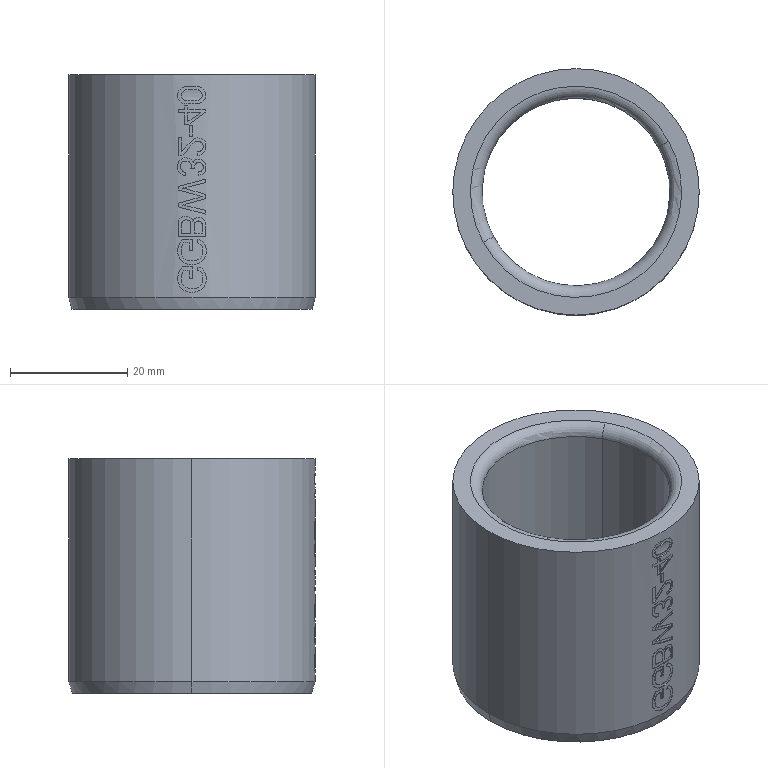Part | STEP file | PN_0055_id1202_x_t | 1 solid | 169 faces | box 42 x 42 x 40 mm | volume 22994 mm3 | plane 104 | cylinder 59 | torus 4 | cone 2 | commonest cylinder face diameters 41.8 x9 42 x6 2.34 x2 2.758 x2 3.023 x2 3.15 x2